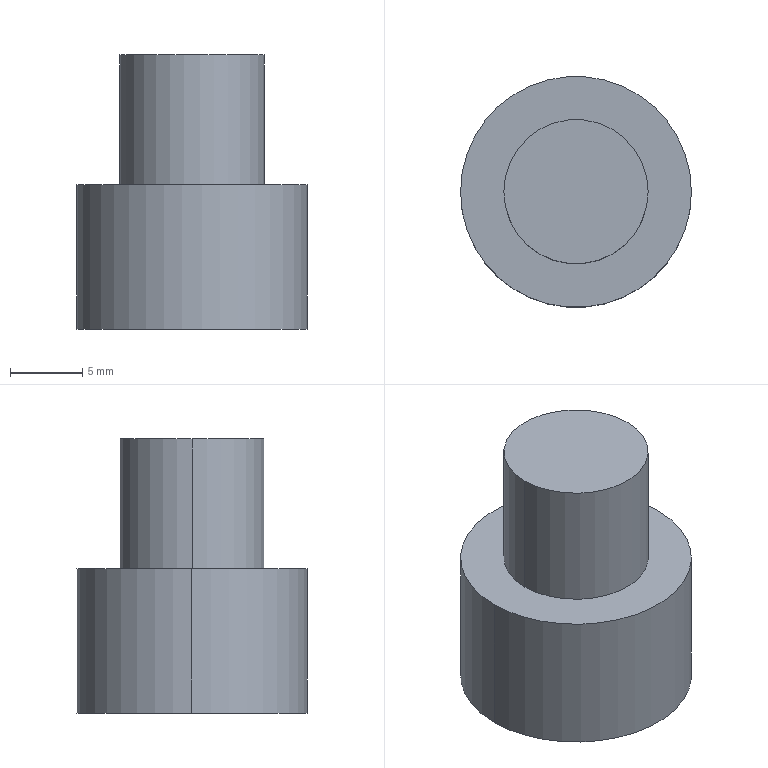Part | STEP file | LG M10_1F | 1 solid | 14 faces | box 16 x 16 x 19 mm | volume 2438 mm3 | plane 10 | cylinder 4 | commonest cylinder face diameters 10 x2 16 x2
STEP:
#1=CARTESIAN_POINT('',(0.,0.,0.));
#2=DIRECTION('',(0.,0.,1.));
#3=DIRECTION('',(1.,0.,0.));
#4=AXIS2_PLACEMENT_3D('',#1,#2,#3);
#5=CARTESIAN_POINT('',(5.,0.,9.));
#6=VERTEX_POINT('',#5);
#7=CARTESIAN_POINT('',(-5.,0.,9.));
#8=VERTEX_POINT('',#7);
#9=CARTESIAN_POINT('',(0.,0.,9.));
#10=DIRECTION('',(0.,0.,1.));
#11=DIRECTION('',(1.,0.,0.));
#12=AXIS2_PLACEMENT_3D('',#9,#10,#11);
#13=CIRCLE('',#12,5.);
#14=CARTESIAN_POINT('',(0.,0.,9.));
#15=DIRECTION('',(0.,0.,-1.));
#16=DIRECTION('',(-1.,0.,0.));
#17=AXIS2_PLACEMENT_3D('',#14,#15,#16);
#18=CYLINDRICAL_SURFACE('',#17,5.);
#19=CARTESIAN_POINT('',(3.142,0.));
#20=DIRECTION('',(-1.,0.));
#21=VECTOR('',#20,1.);
#22=LINE('',#19,#21);
#23=(GEOMETRIC_REPRESENTATION_CONTEXT(2)PARAMETRIC_REPRESENTATION_CONTEXT()REPRESENTATION_CONTEXT('',''));
#24=DEFINITIONAL_REPRESENTATION('',(#22),#23);
#25=PCURVE('',#18,#24);
#26=CARTESIAN_POINT('',(0.,0.,9.));
#27=DIRECTION('',(0.,0.,1.));
#28=DIRECTION('',(1.,0.,0.));
#29=AXIS2_PLACEMENT_3D('',#26,#27,#28);
#30=PLANE('',#29);
#31=CARTESIAN_POINT('',(0.,0.));
#32=DIRECTION('',(1.,0.));
#33=AXIS2_PLACEMENT_2D('',#31,#32);
#34=CIRCLE('',#33,5.);
#35=(GEOMETRIC_REPRESENTATION_CONTEXT(2)PARAMETRIC_REPRESENTATION_CONTEXT()REPRESENTATION_CONTEXT('',''));
#36=DEFINITIONAL_REPRESENTATION('',(#34),#35);
#37=PCURVE('',#30,#36);
#38=SURFACE_CURVE('',#13,(#25,#37),.PCURVE_S1.);
#39=EDGE_CURVE('',#6,#8,#38,.T.);
#40=ORIENTED_EDGE('',*,*,#39,.F.);
#41=CARTESIAN_POINT('',(5.,0.,0.));
#42=VERTEX_POINT('',#41);
#43=CARTESIAN_POINT('',(5.,0.,9.));
#44=DIRECTION('',(0.,0.,-1.));
#45=VECTOR('',#44,1.);
#46=LINE('',#43,#45);
#47=CARTESIAN_POINT('',(3.142,0.));
#48=DIRECTION('',(0.,1.));
#49=VECTOR('',#48,1.);
#50=LINE('',#47,#49);
#51=(GEOMETRIC_REPRESENTATION_CONTEXT(2)PARAMETRIC_REPRESENTATION_CONTEXT()REPRESENTATION_CONTEXT('',''));
#52=DEFINITIONAL_REPRESENTATION('',(#50),#51);
#53=PCURVE('',#18,#52);
#54=CARTESIAN_POINT('',(0.,0.,9.));
#55=DIRECTION('',(0.,0.,-1.));
#56=DIRECTION('',(-1.,0.,0.));
#57=AXIS2_PLACEMENT_3D('',#54,#55,#56);
#58=CYLINDRICAL_SURFACE('',#57,5.);
#59=CARTESIAN_POINT('',(3.142,0.));
#60=DIRECTION('',(0.,1.));
#61=VECTOR('',#60,1.);
#62=LINE('',#59,#61);
#63=(GEOMETRIC_REPRESENTATION_CONTEXT(2)PARAMETRIC_REPRESENTATION_CONTEXT()REPRESENTATION_CONTEXT('',''));
#64=DEFINITIONAL_REPRESENTATION('',(#62),#63);
#65=PCURVE('',#58,#64);
#66=SURFACE_CURVE('',#46,(#53,#65),.PCURVE_S1.);
#67=EDGE_CURVE('',#6,#42,#66,.T.);
#68=ORIENTED_EDGE('',*,*,#67,.T.);
#69=CARTESIAN_POINT('',(-5.,0.,0.));
#70=VERTEX_POINT('',#69);
#71=CARTESIAN_POINT('',(0.,0.,0.));
#72=DIRECTION('',(0.,0.,1.));
#73=DIRECTION('',(1.,0.,0.));
#74=AXIS2_PLACEMENT_3D('',#71,#72,#73);
#75=CIRCLE('',#74,5.);
#76=CARTESIAN_POINT('',(3.142,9.));
#77=DIRECTION('',(-1.,0.));
#78=VECTOR('',#77,1.);
#79=LINE('',#76,#78);
#80=(GEOMETRIC_REPRESENTATION_CONTEXT(2)PARAMETRIC_REPRESENTATION_CONTEXT()REPRESENTATION_CONTEXT('',''));
#81=DEFINITIONAL_REPRESENTATION('',(#79),#80);
#82=PCURVE('',#18,#81);
#83=CARTESIAN_POINT('',(0.,0.,0.));
#84=DIRECTION('',(0.,0.,1.));
#85=DIRECTION('',(1.,0.,0.));
#86=AXIS2_PLACEMENT_3D('',#83,#84,#85);
#87=PLANE('',#86);
#88=CARTESIAN_POINT('',(0.,0.));
#89=DIRECTION('',(1.,0.));
#90=AXIS2_PLACEMENT_2D('',#88,#89);
#91=CIRCLE('',#90,5.);
#92=(GEOMETRIC_REPRESENTATION_CONTEXT(2)PARAMETRIC_REPRESENTATION_CONTEXT()REPRESENTATION_CONTEXT('',''));
#93=DEFINITIONAL_REPRESENTATION('',(#91),#92);
#94=PCURVE('',#87,#93);
#95=SURFACE_CURVE('',#75,(#82,#94),.PCURVE_S1.);
#96=EDGE_CURVE('',#42,#70,#95,.T.);
#97=ORIENTED_EDGE('',*,*,#96,.T.);
#98=CARTESIAN_POINT('',(-5.,0.,9.));
#99=DIRECTION('',(0.,0.,-1.));
#100=VECTOR('',#99,1.);
#101=LINE('',#98,#100);
#102=CARTESIAN_POINT('',(0.,0.));
#103=DIRECTION('',(0.,1.));
#104=VECTOR('',#103,1.);
#105=LINE('',#102,#104);
#106=(GEOMETRIC_REPRESENTATION_CONTEXT(2)PARAMETRIC_REPRESENTATION_CONTEXT()REPRESENTATION_CONTEXT('',''));
#107=DEFINITIONAL_REPRESENTATION('',(#105),#106);
#108=PCURVE('',#18,#107);
#109=CARTESIAN_POINT('',(6.283,0.));
#110=DIRECTION('',(0.,1.));
#111=VECTOR('',#110,1.);
#112=LINE('',#109,#111);
#113=(GEOMETRIC_REPRESENTATION_CONTEXT(2)PARAMETRIC_REPRESENTATION_CONTEXT()REPRESENTATION_CONTEXT('',''));
#114=DEFINITIONAL_REPRESENTATION('',(#112),#113);
#115=PCURVE('',#58,#114);
#116=SURFACE_CURVE('',#101,(#108,#115),.PCURVE_S1.);
#117=EDGE_CURVE('',#8,#70,#116,.T.);
#118=ORIENTED_EDGE('',*,*,#117,.F.);
#119=EDGE_LOOP('',(#40,#68,#97,#118));
#120=FACE_BOUND('',#119,.T.);
#121=ADVANCED_FACE('',(#120),#18,.T.);
#122=CARTESIAN_POINT('',(8.,0.,-10.));
#123=VERTEX_POINT('',#122);
#124=CARTESIAN_POINT('',(-8.,0.,-10.));
#125=VERTEX_POINT('',#124);
#126=CARTESIAN_POINT('',(0.,0.,-10.));
#127=DIRECTION('',(0.,0.,1.));
#128=DIRECTION('',(1.,0.,0.));
#129=AXIS2_PLACEMENT_3D('',#126,#127,#128);
#130=CIRCLE('',#129,8.);
#131=CARTESIAN_POINT('',(0.,0.,-10.));
#132=DIRECTION('',(0.,0.,1.));
#133=DIRECTION('',(1.,0.,0.));
#134=AXIS2_PLACEMENT_3D('',#131,#132,#133);
#135=CYLINDRICAL_SURFACE('',#134,8.);
#136=CARTESIAN_POINT('',(0.,0.));
#137=DIRECTION('',(1.,0.));
#138=VECTOR('',#137,1.);
#139=LINE('',#136,#138);
#140=(GEOMETRIC_REPRESENTATION_CONTEXT(2)PARAMETRIC_REPRESENTATION_CONTEXT()REPRESENTATION_CONTEXT('',''));
#141=DEFINITIONAL_REPRESENTATION('',(#139),#140);
#142=PCURVE('',#135,#141);
#143=CARTESIAN_POINT('',(0.,0.,-10.));
#144=DIRECTION('',(0.,0.,1.));
#145=DIRECTION('',(1.,0.,0.));
#146=AXIS2_PLACEMENT_3D('',#143,#144,#145);
#147=PLANE('',#146);
#148=CARTESIAN_POINT('',(0.,0.));
#149=DIRECTION('',(1.,0.));
#150=AXIS2_PLACEMENT_2D('',#148,#149);
#151=CIRCLE('',#150,8.);
#152=(GEOMETRIC_REPRESENTATION_CONTEXT(2)PARAMETRIC_REPRESENTATION_CONTEXT()REPRESENTATION_CONTEXT('',''));
#153=DEFINITIONAL_REPRESENTATION('',(#151),#152);
#154=PCURVE('',#147,#153);
#155=SURFACE_CURVE('',#130,(#142,#154),.PCURVE_S1.);
#156=EDGE_CURVE('',#123,#125,#155,.T.);
#157=ORIENTED_EDGE('',*,*,#156,.T.);
#158=CARTESIAN_POINT('',(-8.,0.,0.));
#159=VERTEX_POINT('',#158);
#160=CARTESIAN_POINT('',(-8.,0.,-10.));
#161=DIRECTION('',(0.,0.,1.));
#162=VECTOR('',#161,1.);
#163=LINE('',#160,#162);
#164=CARTESIAN_POINT('',(3.142,0.));
#165=DIRECTION('',(0.,1.));
#166=VECTOR('',#165,1.);
#167=LINE('',#164,#166);
#168=(GEOMETRIC_REPRESENTATION_CONTEXT(2)PARAMETRIC_REPRESENTATION_CONTEXT()REPRESENTATION_CONTEXT('',''));
#169=DEFINITIONAL_REPRESENTATION('',(#167),#168);
#170=PCURVE('',#135,#169);
#171=CARTESIAN_POINT('',(0.,0.,-10.));
#172=DIRECTION('',(0.,0.,1.));
#173=DIRECTION('',(1.,0.,0.));
#174=AXIS2_PLACEMENT_3D('',#171,#172,#173);
#175=CYLINDRICAL_SURFACE('',#174,8.);
#176=CARTESIAN_POINT('',(3.142,0.));
#177=DIRECTION('',(0.,1.));
#178=VECTOR('',#177,1.);
#179=LINE('',#176,#178);
#180=(GEOMETRIC_REPRESENTATION_CONTEXT(2)PARAMETRIC_REPRESENTATION_CONTEXT()REPRESENTATION_CONTEXT('',''));
#181=DEFINITIONAL_REPRESENTATION('',(#179),#180);
#182=PCURVE('',#175,#181);
#183=SURFACE_CURVE('',#163,(#170,#182),.PCURVE_S1.);
#184=EDGE_CURVE('',#125,#159,#183,.T.);
#185=ORIENTED_EDGE('',*,*,#184,.T.);
#186=CARTESIAN_POINT('',(8.,0.,0.));
#187=VERTEX_POINT('',#186);
#188=CARTESIAN_POINT('',(0.,0.,0.));
#189=DIRECTION('',(0.,0.,1.));
#190=DIRECTION('',(1.,0.,0.));
#191=AXIS2_PLACEMENT_3D('',#188,#189,#190);
#192=CIRCLE('',#191,8.);
#193=CARTESIAN_POINT('',(0.,10.));
#194=DIRECTION('',(1.,0.));
#195=VECTOR('',#194,1.);
#196=LINE('',#193,#195);
#197=(GEOMETRIC_REPRESENTATION_CONTEXT(2)PARAMETRIC_REPRESENTATION_CONTEXT()REPRESENTATION_CONTEXT('',''));
#198=DEFINITIONAL_REPRESENTATION('',(#196),#197);
#199=PCURVE('',#135,#198);
#200=CARTESIAN_POINT('',(0.,0.));
#201=DIRECTION('',(1.,0.));
#202=AXIS2_PLACEMENT_2D('',#200,#201);
#203=CIRCLE('',#202,8.);
#204=(GEOMETRIC_REPRESENTATION_CONTEXT(2)PARAMETRIC_REPRESENTATION_CONTEXT()REPRESENTATION_CONTEXT('',''));
#205=DEFINITIONAL_REPRESENTATION('',(#203),#204);
#206=PCURVE('',#87,#205);
#207=SURFACE_CURVE('',#192,(#199,#206),.PCURVE_S1.);
#208=EDGE_CURVE('',#187,#159,#207,.T.);
#209=ORIENTED_EDGE('',*,*,#208,.F.);
#210=CARTESIAN_POINT('',(8.,0.,-10.));
#211=DIRECTION('',(0.,0.,1.));
#212=VECTOR('',#211,1.);
#213=LINE('',#210,#212);
#214=CARTESIAN_POINT('',(0.,0.));
#215=DIRECTION('',(0.,1.));
#216=VECTOR('',#215,1.);
#217=LINE('',#214,#216);
#218=(GEOMETRIC_REPRESENTATION_CONTEXT(2)PARAMETRIC_REPRESENTATION_CONTEXT()REPRESENTATION_CONTEXT('',''));
#219=DEFINITIONAL_REPRESENTATION('',(#217),#218);
#220=PCURVE('',#135,#219);
#221=CARTESIAN_POINT('',(6.283,0.));
#222=DIRECTION('',(0.,1.));
#223=VECTOR('',#222,1.);
#224=LINE('',#221,#223);
#225=(GEOMETRIC_REPRESENTATION_CONTEXT(2)PARAMETRIC_REPRESENTATION_CONTEXT()REPRESENTATION_CONTEXT('',''));
#226=DEFINITIONAL_REPRESENTATION('',(#224),#225);
#227=PCURVE('',#175,#226);
#228=SURFACE_CURVE('',#213,(#220,#227),.PCURVE_S1.);
#229=EDGE_CURVE('',#123,#187,#228,.T.);
#230=ORIENTED_EDGE('',*,*,#229,.F.);
#231=EDGE_LOOP('',(#157,#185,#209,#230));
#232=FACE_BOUND('',#231,.T.);
#233=ADVANCED_FACE('',(#232),#135,.T.);
#234=ORIENTED_EDGE('',*,*,#208,.T.);
#235=CARTESIAN_POINT('',(0.,0.,0.));
#236=DIRECTION('',(0.,0.,1.));
#237=DIRECTION('',(1.,0.,0.));
#238=AXIS2_PLACEMENT_3D('',#235,#236,#237);
#239=CIRCLE('',#238,8.);
#240=CARTESIAN_POINT('',(0.,0.));
#241=DIRECTION('',(1.,0.));
#242=AXIS2_PLACEMENT_2D('',#240,#241);
#243=CIRCLE('',#242,8.);
#244=(GEOMETRIC_REPRESENTATION_CONTEXT(2)PARAMETRIC_REPRESENTATION_CONTEXT()REPRESENTATION_CONTEXT('',''));
#245=DEFINITIONAL_REPRESENTATION('',(#243),#244);
#246=PCURVE('',#87,#245);
#247=CARTESIAN_POINT('',(0.,10.));
#248=DIRECTION('',(1.,0.));
#249=VECTOR('',#248,1.);
#250=LINE('',#247,#249);
#251=(GEOMETRIC_REPRESENTATION_CONTEXT(2)PARAMETRIC_REPRESENTATION_CONTEXT()REPRESENTATION_CONTEXT('',''));
#252=DEFINITIONAL_REPRESENTATION('',(#250),#251);
#253=PCURVE('',#175,#252);
#254=SURFACE_CURVE('',#239,(#246,#253),.PCURVE_S1.);
#255=EDGE_CURVE('',#159,#187,#254,.T.);
#256=ORIENTED_EDGE('',*,*,#255,.T.);
#257=EDGE_LOOP('',(#234,#256));
#258=FACE_BOUND('',#257,.T.);
#259=CARTESIAN_POINT('',(0.,0.,0.));
#260=DIRECTION('',(0.,0.,1.));
#261=DIRECTION('',(1.,0.,0.));
#262=AXIS2_PLACEMENT_3D('',#259,#260,#261);
#263=CIRCLE('',#262,5.);
#264=CARTESIAN_POINT('',(0.,0.));
#265=DIRECTION('',(1.,0.));
#266=AXIS2_PLACEMENT_2D('',#264,#265);
#267=CIRCLE('',#266,5.);
#268=(GEOMETRIC_REPRESENTATION_CONTEXT(2)PARAMETRIC_REPRESENTATION_CONTEXT()REPRESENTATION_CONTEXT('',''));
#269=DEFINITIONAL_REPRESENTATION('',(#267),#268);
#270=PCURVE('',#87,#269);
#271=CARTESIAN_POINT('',(9.425,9.));
#272=DIRECTION('',(-1.,0.));
#273=VECTOR('',#272,1.);
#274=LINE('',#271,#273);
#275=(GEOMETRIC_REPRESENTATION_CONTEXT(2)PARAMETRIC_REPRESENTATION_CONTEXT()REPRESENTATION_CONTEXT('',''));
#276=DEFINITIONAL_REPRESENTATION('',(#274),#275);
#277=PCURVE('',#58,#276);
#278=SURFACE_CURVE('',#263,(#270,#277),.PCURVE_S1.);
#279=EDGE_CURVE('',#70,#42,#278,.T.);
#280=ORIENTED_EDGE('',*,*,#279,.F.);
#281=ORIENTED_EDGE('',*,*,#96,.F.);
#282=EDGE_LOOP('',(#280,#281));
#283=FACE_BOUND('',#282,.T.);
#284=ADVANCED_FACE('',(#258,#283),#87,.T.);
#285=ORIENTED_EDGE('',*,*,#184,.F.);
#286=CARTESIAN_POINT('',(0.,0.,-10.));
#287=DIRECTION('',(0.,0.,1.));
#288=DIRECTION('',(1.,0.,0.));
#289=AXIS2_PLACEMENT_3D('',#286,#287,#288);
#290=CIRCLE('',#289,8.);
#291=CARTESIAN_POINT('',(0.,0.));
#292=DIRECTION('',(1.,0.));
#293=VECTOR('',#292,1.);
#294=LINE('',#291,#293);
#295=(GEOMETRIC_REPRESENTATION_CONTEXT(2)PARAMETRIC_REPRESENTATION_CONTEXT()REPRESENTATION_CONTEXT('',''));
#296=DEFINITIONAL_REPRESENTATION('',(#294),#295);
#297=PCURVE('',#175,#296);
#298=CARTESIAN_POINT('',(0.,0.));
#299=DIRECTION('',(1.,0.));
#300=AXIS2_PLACEMENT_2D('',#298,#299);
#301=CIRCLE('',#300,8.);
#302=(GEOMETRIC_REPRESENTATION_CONTEXT(2)PARAMETRIC_REPRESENTATION_CONTEXT()REPRESENTATION_CONTEXT('',''));
#303=DEFINITIONAL_REPRESENTATION('',(#301),#302);
#304=PCURVE('',#147,#303);
#305=SURFACE_CURVE('',#290,(#297,#304),.PCURVE_S1.);
#306=EDGE_CURVE('',#125,#123,#305,.T.);
#307=ORIENTED_EDGE('',*,*,#306,.T.);
#308=ORIENTED_EDGE('',*,*,#229,.T.);
#309=ORIENTED_EDGE('',*,*,#255,.F.);
#310=EDGE_LOOP('',(#285,#307,#308,#309));
#311=FACE_BOUND('',#310,.T.);
#312=ADVANCED_FACE('',(#311),#175,.T.);
#313=CARTESIAN_POINT('',(-4.636,0.,-10.));
#314=VERTEX_POINT('',#313);
#315=CARTESIAN_POINT('',(-2.318,4.015,-10.));
#316=VERTEX_POINT('',#315);
#317=CARTESIAN_POINT('',(-4.636,0.,-10.));
#318=DIRECTION('',(0.5,0.866,0.));
#319=VECTOR('',#318,1.);
#320=LINE('',#317,#319);
#321=CARTESIAN_POINT('',(-4.636,0.));
#322=DIRECTION('',(0.5,0.866));
#323=VECTOR('',#322,1.);
#324=LINE('',#321,#323);
#325=(GEOMETRIC_REPRESENTATION_CONTEXT(2)PARAMETRIC_REPRESENTATION_CONTEXT()REPRESENTATION_CONTEXT('',''));
#326=DEFINITIONAL_REPRESENTATION('',(#324),#325);
#327=PCURVE('',#147,#326);
#328=CARTESIAN_POINT('',(-4.636,0.,-5.));
#329=DIRECTION('',(-0.866,0.5,0.));
#330=DIRECTION('',(-0.5,-0.866,0.));
#331=AXIS2_PLACEMENT_3D('',#328,#329,#330);
#332=PLANE('',#331);
#333=CARTESIAN_POINT('',(0.,-5.));
#334=DIRECTION('',(-1.,0.));
#335=VECTOR('',#334,1.);
#336=LINE('',#333,#335);
#337=(GEOMETRIC_REPRESENTATION_CONTEXT(2)PARAMETRIC_REPRESENTATION_CONTEXT()REPRESENTATION_CONTEXT('',''));
#338=DEFINITIONAL_REPRESENTATION('',(#336),#337);
#339=PCURVE('',#332,#338);
#340=SURFACE_CURVE('',#320,(#327,#339),.PCURVE_S1.);
#341=EDGE_CURVE('',#314,#316,#340,.T.);
#342=ORIENTED_EDGE('',*,*,#341,.F.);
#343=CARTESIAN_POINT('',(-2.318,-4.015,-10.));
#344=VERTEX_POINT('',#343);
#345=CARTESIAN_POINT('',(-2.318,-4.015,-10.));
#346=DIRECTION('',(-0.5,0.866,0.));
#347=VECTOR('',#346,1.);
#348=LINE('',#345,#347);
#349=CARTESIAN_POINT('',(-2.318,-4.015));
#350=DIRECTION('',(-0.5,0.866));
#351=VECTOR('',#350,1.);
#352=LINE('',#349,#351);
#353=(GEOMETRIC_REPRESENTATION_CONTEXT(2)PARAMETRIC_REPRESENTATION_CONTEXT()REPRESENTATION_CONTEXT('',''));
#354=DEFINITIONAL_REPRESENTATION('',(#352),#353);
#355=PCURVE('',#147,#354);
#356=CARTESIAN_POINT('',(-2.318,-4.015,-5.));
#357=DIRECTION('',(-0.866,-0.5,0.));
#358=DIRECTION('',(0.5,-0.866,0.));
#359=AXIS2_PLACEMENT_3D('',#356,#357,#358);
#360=PLANE('',#359);
#361=CARTESIAN_POINT('',(0.,-5.));
#362=DIRECTION('',(-1.,0.));
#363=VECTOR('',#362,1.);
#364=LINE('',#361,#363);
#365=(GEOMETRIC_REPRESENTATION_CONTEXT(2)PARAMETRIC_REPRESENTATION_CONTEXT()REPRESENTATION_CONTEXT('',''));
#366=DEFINITIONAL_REPRESENTATION('',(#364),#365);
#367=PCURVE('',#360,#366);
#368=SURFACE_CURVE('',#348,(#355,#367),.PCURVE_S1.);
#369=EDGE_CURVE('',#344,#314,#368,.T.);
#370=ORIENTED_EDGE('',*,*,#369,.F.);
#371=CARTESIAN_POINT('',(2.318,-4.015,-10.));
#372=VERTEX_POINT('',#371);
#373=CARTESIAN_POINT('',(2.318,-4.015,-10.));
#374=DIRECTION('',(-1.,0.,0.));
#375=VECTOR('',#374,1.);
#376=LINE('',#373,#375);
#377=CARTESIAN_POINT('',(2.318,-4.015));
#378=DIRECTION('',(-1.,0.));
#379=VECTOR('',#378,1.);
#380=LINE('',#377,#379);
#381=(GEOMETRIC_REPRESENTATION_CONTEXT(2)PARAMETRIC_REPRESENTATION_CONTEXT()REPRESENTATION_CONTEXT('',''));
#382=DEFINITIONAL_REPRESENTATION('',(#380),#381);
#383=PCURVE('',#147,#382);
#384=CARTESIAN_POINT('',(2.318,-4.015,-5.));
#385=DIRECTION('',(0.,-1.,0.));
#386=DIRECTION('',(1.,0.,0.));
#387=AXIS2_PLACEMENT_3D('',#384,#385,#386);
#388=PLANE('',#387);
#389=CARTESIAN_POINT('',(0.,-5.));
#390=DIRECTION('',(-1.,0.));
#391=VECTOR('',#390,1.);
#392=LINE('',#389,#391);
#393=(GEOMETRIC_REPRESENTATION_CONTEXT(2)PARAMETRIC_REPRESENTATION_CONTEXT()REPRESENTATION_CONTEXT('',''));
#394=DEFINITIONAL_REPRESENTATION('',(#392),#393);
#395=PCURVE('',#388,#394);
#396=SURFACE_CURVE('',#376,(#383,#395),.PCURVE_S1.);
#397=EDGE_CURVE('',#372,#344,#396,.T.);
#398=ORIENTED_EDGE('',*,*,#397,.F.);
#399=CARTESIAN_POINT('',(4.636,0.,-10.));
#400=VERTEX_POINT('',#399);
#401=CARTESIAN_POINT('',(4.636,0.,-10.));
#402=DIRECTION('',(-0.5,-0.866,0.));
#403=VECTOR('',#402,1.);
#404=LINE('',#401,#403);
#405=CARTESIAN_POINT('',(4.636,0.));
#406=DIRECTION('',(-0.5,-0.866));
#407=VECTOR('',#406,1.);
#408=LINE('',#405,#407);
#409=(GEOMETRIC_REPRESENTATION_CONTEXT(2)PARAMETRIC_REPRESENTATION_CONTEXT()REPRESENTATION_CONTEXT('',''));
#410=DEFINITIONAL_REPRESENTATION('',(#408),#409);
#411=PCURVE('',#147,#410);
#412=CARTESIAN_POINT('',(4.636,0.,-5.));
#413=DIRECTION('',(0.866,-0.5,0.));
#414=DIRECTION('',(0.5,0.866,0.));
#415=AXIS2_PLACEMENT_3D('',#412,#413,#414);
#416=PLANE('',#415);
#417=CARTESIAN_POINT('',(0.,-5.));
#418=DIRECTION('',(-1.,0.));
#419=VECTOR('',#418,1.);
#420=LINE('',#417,#419);
#421=(GEOMETRIC_REPRESENTATION_CONTEXT(2)PARAMETRIC_REPRESENTATION_CONTEXT()REPRESENTATION_CONTEXT('',''));
#422=DEFINITIONAL_REPRESENTATION('',(#420),#421);
#423=PCURVE('',#416,#422);
#424=SURFACE_CURVE('',#404,(#411,#423),.PCURVE_S1.);
#425=EDGE_CURVE('',#400,#372,#424,.T.);
#426=ORIENTED_EDGE('',*,*,#425,.F.);
#427=CARTESIAN_POINT('',(2.318,4.015,-10.));
#428=VERTEX_POINT('',#427);
#429=CARTESIAN_POINT('',(2.318,4.015,-10.));
#430=DIRECTION('',(0.5,-0.866,0.));
#431=VECTOR('',#430,1.);
#432=LINE('',#429,#431);
#433=CARTESIAN_POINT('',(2.318,4.015));
#434=DIRECTION('',(0.5,-0.866));
#435=VECTOR('',#434,1.);
#436=LINE('',#433,#435);
#437=(GEOMETRIC_REPRESENTATION_CONTEXT(2)PARAMETRIC_REPRESENTATION_CONTEXT()REPRESENTATION_CONTEXT('',''));
#438=DEFINITIONAL_REPRESENTATION('',(#436),#437);
#439=PCURVE('',#147,#438);
#440=CARTESIAN_POINT('',(2.318,4.015,-5.));
#441=DIRECTION('',(0.866,0.5,0.));
#442=DIRECTION('',(-0.5,0.866,0.));
#443=AXIS2_PLACEMENT_3D('',#440,#441,#442);
#444=PLANE('',#443);
#445=CARTESIAN_POINT('',(0.,-5.));
#446=DIRECTION('',(-1.,0.));
#447=VECTOR('',#446,1.);
#448=LINE('',#445,#447);
#449=(GEOMETRIC_REPRESENTATION_CONTEXT(2)PARAMETRIC_REPRESENTATION_CONTEXT()REPRESENTATION_CONTEXT('',''));
#450=DEFINITIONAL_REPRESENTATION('',(#448),#449);
#451=PCURVE('',#444,#450);
#452=SURFACE_CURVE('',#432,(#439,#451),.PCURVE_S1.);
#453=EDGE_CURVE('',#428,#400,#452,.T.);
#454=ORIENTED_EDGE('',*,*,#453,.F.);
#455=CARTESIAN_POINT('',(-2.318,4.015,-10.));
#456=DIRECTION('',(1.,0.,0.));
#457=VECTOR('',#456,1.);
#458=LINE('',#455,#457);
#459=CARTESIAN_POINT('',(-2.318,4.015));
#460=DIRECTION('',(1.,0.));
#461=VECTOR('',#460,1.);
#462=LINE('',#459,#461);
#463=(GEOMETRIC_REPRESENTATION_CONTEXT(2)PARAMETRIC_REPRESENTATION_CONTEXT()REPRESENTATION_CONTEXT('',''));
#464=DEFINITIONAL_REPRESENTATION('',(#462),#463);
#465=PCURVE('',#147,#464);
#466=CARTESIAN_POINT('',(-2.318,4.015,-5.));
#467=DIRECTION('',(0.,1.,0.));
#468=DIRECTION('',(-1.,0.,0.));
#469=AXIS2_PLACEMENT_3D('',#466,#467,#468);
#470=PLANE('',#469);
#471=CARTESIAN_POINT('',(0.,-5.));
#472=DIRECTION('',(-1.,0.));
#473=VECTOR('',#472,1.);
#474=LINE('',#471,#473);
#475=(GEOMETRIC_REPRESENTATION_CONTEXT(2)PARAMETRIC_REPRESENTATION_CONTEXT()REPRESENTATION_CONTEXT('',''));
#476=DEFINITIONAL_REPRESENTATION('',(#474),#475);
#477=PCURVE('',#470,#476);
#478=SURFACE_CURVE('',#458,(#465,#477),.PCURVE_S1.);
#479=EDGE_CURVE('',#316,#428,#478,.T.);
#480=ORIENTED_EDGE('',*,*,#479,.F.);
#481=EDGE_LOOP('',(#342,#370,#398,#426,#454,#480));
#482=FACE_BOUND('',#481,.T.);
#483=ORIENTED_EDGE('',*,*,#156,.F.);
#484=ORIENTED_EDGE('',*,*,#306,.F.);
#485=EDGE_LOOP('',(#483,#484));
#486=FACE_BOUND('',#485,.T.);
#487=ADVANCED_FACE('',(#482,#486),#147,.F.);
#488=ORIENTED_EDGE('',*,*,#67,.F.);
#489=CARTESIAN_POINT('',(0.,0.,9.));
#490=DIRECTION('',(0.,0.,1.));
#491=DIRECTION('',(1.,0.,0.));
#492=AXIS2_PLACEMENT_3D('',#489,#490,#491);
#493=CIRCLE('',#492,5.);
#494=CARTESIAN_POINT('',(9.425,0.));
#495=DIRECTION('',(-1.,0.));
#496=VECTOR('',#495,1.);
#497=LINE('',#494,#496);
#498=(GEOMETRIC_REPRESENTATION_CONTEXT(2)PARAMETRIC_REPRESENTATION_CONTEXT()REPRESENTATION_CONTEXT('',''));
#499=DEFINITIONAL_REPRESENTATION('',(#497),#498);
#500=PCURVE('',#58,#499);
#501=CARTESIAN_POINT('',(0.,0.));
#502=DIRECTION('',(1.,0.));
#503=AXIS2_PLACEMENT_2D('',#501,#502);
#504=CIRCLE('',#503,5.);
#505=(GEOMETRIC_REPRESENTATION_CONTEXT(2)PARAMETRIC_REPRESENTATION_CONTEXT()REPRESENTATION_CONTEXT('',''));
#506=DEFINITIONAL_REPRESENTATION('',(#504),#505);
#507=PCURVE('',#30,#506);
#508=SURFACE_CURVE('',#493,(#500,#507),.PCURVE_S1.);
#509=EDGE_CURVE('',#8,#6,#508,.T.);
#510=ORIENTED_EDGE('',*,*,#509,.F.);
#511=ORIENTED_EDGE('',*,*,#117,.T.);
#512=ORIENTED_EDGE('',*,*,#279,.T.);
#513=EDGE_LOOP('',(#488,#510,#511,#512));
#514=FACE_BOUND('',#513,.T.);
#515=ADVANCED_FACE('',(#514),#58,.T.);
#516=ORIENTED_EDGE('',*,*,#509,.T.);
#517=ORIENTED_EDGE('',*,*,#39,.T.);
#518=EDGE_LOOP('',(#516,#517));
#519=FACE_BOUND('',#518,.T.);
#520=ADVANCED_FACE('',(#519),#30,.T.);
#521=ORIENTED_EDGE('',*,*,#369,.T.);
#522=CARTESIAN_POINT('',(-4.636,0.,-5.));
#523=VERTEX_POINT('',#522);
#524=CARTESIAN_POINT('',(-4.636,0.,-5.));
#525=DIRECTION('',(0.,0.,-1.));
#526=VECTOR('',#525,1.);
#527=LINE('',#524,#526);
#528=CARTESIAN_POINT('',(-4.636,0.));
#529=DIRECTION('',(0.,-1.));
#530=VECTOR('',#529,1.);
#531=LINE('',#528,#530);
#532=(GEOMETRIC_REPRESENTATION_CONTEXT(2)PARAMETRIC_REPRESENTATION_CONTEXT()REPRESENTATION_CONTEXT('',''));
#533=DEFINITIONAL_REPRESENTATION('',(#531),#532);
#534=PCURVE('',#360,#533);
#535=CARTESIAN_POINT('',(0.,0.));
#536=DIRECTION('',(0.,-1.));
#537=VECTOR('',#536,1.);
#538=LINE('',#535,#537);
#539=(GEOMETRIC_REPRESENTATION_CONTEXT(2)PARAMETRIC_REPRESENTATION_CONTEXT()REPRESENTATION_CONTEXT('',''));
#540=DEFINITIONAL_REPRESENTATION('',(#538),#539);
#541=PCURVE('',#332,#540);
#542=SURFACE_CURVE('',#527,(#534,#541),.PCURVE_S1.);
#543=EDGE_CURVE('',#523,#314,#542,.T.);
#544=ORIENTED_EDGE('',*,*,#543,.F.);
#545=CARTESIAN_POINT('',(-2.318,-4.015,-5.));
#546=VERTEX_POINT('',#545);
#547=CARTESIAN_POINT('',(-2.318,-4.015,-5.));
#548=DIRECTION('',(-0.5,0.866,0.));
#549=VECTOR('',#548,1.);
#550=LINE('',#547,#549);
#551=CARTESIAN_POINT('',(0.,0.));
#552=DIRECTION('',(-1.,0.));
#553=VECTOR('',#552,1.);
#554=LINE('',#551,#553);
#555=(GEOMETRIC_REPRESENTATION_CONTEXT(2)PARAMETRIC_REPRESENTATION_CONTEXT()REPRESENTATION_CONTEXT('',''));
#556=DEFINITIONAL_REPRESENTATION('',(#554),#555);
#557=PCURVE('',#360,#556);
#558=CARTESIAN_POINT('',(0.,0.,-5.));
#559=DIRECTION('',(0.,0.,-1.));
#560=DIRECTION('',(-1.,0.,0.));
#561=AXIS2_PLACEMENT_3D('',#558,#559,#560);
#562=PLANE('',#561);
#563=CARTESIAN_POINT('',(2.318,-4.015));
#564=DIRECTION('',(0.5,0.866));
#565=VECTOR('',#564,1.);
#566=LINE('',#563,#565);
#567=(GEOMETRIC_REPRESENTATION_CONTEXT(2)PARAMETRIC_REPRESENTATION_CONTEXT()REPRESENTATION_CONTEXT('',''));
#568=DEFINITIONAL_REPRESENTATION('',(#566),#567);
#569=PCURVE('',#562,#568);
#570=SURFACE_CURVE('',#550,(#557,#569),.PCURVE_S1.);
#571=EDGE_CURVE('',#546,#523,#570,.T.);
#572=ORIENTED_EDGE('',*,*,#571,.F.);
#573=CARTESIAN_POINT('',(-2.318,-4.015,-5.));
#574=DIRECTION('',(0.,0.,-1.));
#575=VECTOR('',#574,1.);
#576=LINE('',#573,#575);
#577=CARTESIAN_POINT('',(0.,0.));
#578=DIRECTION('',(0.,-1.));
#579=VECTOR('',#578,1.);
#580=LINE('',#577,#579);
#581=(GEOMETRIC_REPRESENTATION_CONTEXT(2)PARAMETRIC_REPRESENTATION_CONTEXT()REPRESENTATION_CONTEXT('',''));
#582=DEFINITIONAL_REPRESENTATION('',(#580),#581);
#583=PCURVE('',#360,#582);
#584=CARTESIAN_POINT('',(-4.636,0.));
#585=DIRECTION('',(0.,-1.));
#586=VECTOR('',#585,1.);
#587=LINE('',#584,#586);
#588=(GEOMETRIC_REPRESENTATION_CONTEXT(2)PARAMETRIC_REPRESENTATION_CONTEXT()REPRESENTATION_CONTEXT('',''));
#589=DEFINITIONAL_REPRESENTATION('',(#587),#588);
#590=PCURVE('',#388,#589);
#591=SURFACE_CURVE('',#576,(#583,#590),.PCURVE_S1.);
#592=EDGE_CURVE('',#546,#344,#591,.T.);
#593=ORIENTED_EDGE('',*,*,#592,.T.);
#594=EDGE_LOOP('',(#521,#544,#572,#593));
#595=FACE_BOUND('',#594,.T.);
#596=ADVANCED_FACE('',(#595),#360,.F.);
#597=ORIENTED_EDGE('',*,*,#397,.T.);
#598=ORIENTED_EDGE('',*,*,#592,.F.);
#599=CARTESIAN_POINT('',(2.318,-4.015,-5.));
#600=VERTEX_POINT('',#599);
#601=CARTESIAN_POINT('',(2.318,-4.015,-5.));
#602=DIRECTION('',(-1.,0.,0.));
#603=VECTOR('',#602,1.);
#604=LINE('',#601,#603);
#605=CARTESIAN_POINT('',(0.,0.));
#606=DIRECTION('',(-1.,0.));
#607=VECTOR('',#606,1.);
#608=LINE('',#605,#607);
#609=(GEOMETRIC_REPRESENTATION_CONTEXT(2)PARAMETRIC_REPRESENTATION_CONTEXT()REPRESENTATION_CONTEXT('',''));
#610=DEFINITIONAL_REPRESENTATION('',(#608),#609);
#611=PCURVE('',#388,#610);
#612=CARTESIAN_POINT('',(-2.318,-4.015));
#613=DIRECTION('',(1.,0.));
#614=VECTOR('',#613,1.);
#615=LINE('',#612,#614);
#616=(GEOMETRIC_REPRESENTATION_CONTEXT(2)PARAMETRIC_REPRESENTATION_CONTEXT()REPRESENTATION_CONTEXT('',''));
#617=DEFINITIONAL_REPRESENTATION('',(#615),#616);
#618=PCURVE('',#562,#617);
#619=SURFACE_CURVE('',#604,(#611,#618),.PCURVE_S1.);
#620=EDGE_CURVE('',#600,#546,#619,.T.);
#621=ORIENTED_EDGE('',*,*,#620,.F.);
#622=CARTESIAN_POINT('',(2.318,-4.015,-5.));
#623=DIRECTION('',(0.,0.,-1.));
#624=VECTOR('',#623,1.);
#625=LINE('',#622,#624);
#626=CARTESIAN_POINT('',(0.,0.));
#627=DIRECTION('',(0.,-1.));
#628=VECTOR('',#627,1.);
#629=LINE('',#626,#628);
#630=(GEOMETRIC_REPRESENTATION_CONTEXT(2)PARAMETRIC_REPRESENTATION_CONTEXT()REPRESENTATION_CONTEXT('',''));
#631=DEFINITIONAL_REPRESENTATION('',(#629),#630);
#632=PCURVE('',#388,#631);
#633=CARTESIAN_POINT('',(-4.636,0.));
#634=DIRECTION('',(0.,-1.));
#635=VECTOR('',#634,1.);
#636=LINE('',#633,#635);
#637=(GEOMETRIC_REPRESENTATION_CONTEXT(2)PARAMETRIC_REPRESENTATION_CONTEXT()REPRESENTATION_CONTEXT('',''));
#638=DEFINITIONAL_REPRESENTATION('',(#636),#637);
#639=PCURVE('',#416,#638);
#640=SURFACE_CURVE('',#625,(#632,#639),.PCURVE_S1.);
#641=EDGE_CURVE('',#600,#372,#640,.T.);
#642=ORIENTED_EDGE('',*,*,#641,.T.);
#643=EDGE_LOOP('',(#597,#598,#621,#642));
#644=FACE_BOUND('',#643,.T.);
#645=ADVANCED_FACE('',(#644),#388,.F.);
#646=ORIENTED_EDGE('',*,*,#425,.T.);
#647=ORIENTED_EDGE('',*,*,#641,.F.);
#648=CARTESIAN_POINT('',(4.636,0.,-5.));
#649=VERTEX_POINT('',#648);
#650=CARTESIAN_POINT('',(4.636,0.,-5.));
#651=DIRECTION('',(-0.5,-0.866,0.));
#652=VECTOR('',#651,1.);
#653=LINE('',#650,#652);
#654=CARTESIAN_POINT('',(0.,0.));
#655=DIRECTION('',(-1.,0.));
#656=VECTOR('',#655,1.);
#657=LINE('',#654,#656);
#658=(GEOMETRIC_REPRESENTATION_CONTEXT(2)PARAMETRIC_REPRESENTATION_CONTEXT()REPRESENTATION_CONTEXT('',''));
#659=DEFINITIONAL_REPRESENTATION('',(#657),#658);
#660=PCURVE('',#416,#659);
#661=CARTESIAN_POINT('',(-4.636,0.));
#662=DIRECTION('',(0.5,-0.866));
#663=VECTOR('',#662,1.);
#664=LINE('',#661,#663);
#665=(GEOMETRIC_REPRESENTATION_CONTEXT(2)PARAMETRIC_REPRESENTATION_CONTEXT()REPRESENTATION_CONTEXT('',''));
#666=DEFINITIONAL_REPRESENTATION('',(#664),#665);
#667=PCURVE('',#562,#666);
#668=SURFACE_CURVE('',#653,(#660,#667),.PCURVE_S1.);
#669=EDGE_CURVE('',#649,#600,#668,.T.);
#670=ORIENTED_EDGE('',*,*,#669,.F.);
#671=CARTESIAN_POINT('',(4.636,0.,-5.));
#672=DIRECTION('',(0.,0.,-1.));
#673=VECTOR('',#672,1.);
#674=LINE('',#671,#673);
#675=CARTESIAN_POINT('',(0.,0.));
#676=DIRECTION('',(0.,-1.));
#677=VECTOR('',#676,1.);
#678=LINE('',#675,#677);
#679=(GEOMETRIC_REPRESENTATION_CONTEXT(2)PARAMETRIC_REPRESENTATION_CONTEXT()REPRESENTATION_CONTEXT('',''));
#680=DEFINITIONAL_REPRESENTATION('',(#678),#679);
#681=PCURVE('',#416,#680);
#682=CARTESIAN_POINT('',(-4.636,0.));
#683=DIRECTION('',(0.,-1.));
#684=VECTOR('',#683,1.);
#685=LINE('',#682,#684);
#686=(GEOMETRIC_REPRESENTATION_CONTEXT(2)PARAMETRIC_REPRESENTATION_CONTEXT()REPRESENTATION_CONTEXT('',''));
#687=DEFINITIONAL_REPRESENTATION('',(#685),#686);
#688=PCURVE('',#444,#687);
#689=SURFACE_CURVE('',#674,(#681,#688),.PCURVE_S1.);
#690=EDGE_CURVE('',#649,#400,#689,.T.);
#691=ORIENTED_EDGE('',*,*,#690,.T.);
#692=EDGE_LOOP('',(#646,#647,#670,#691));
#693=FACE_BOUND('',#692,.T.);
#694=ADVANCED_FACE('',(#693),#416,.F.);
#695=ORIENTED_EDGE('',*,*,#453,.T.);
#696=ORIENTED_EDGE('',*,*,#690,.F.);
#697=CARTESIAN_POINT('',(2.318,4.015,-5.));
#698=VERTEX_POINT('',#697);
#699=CARTESIAN_POINT('',(2.318,4.015,-5.));
#700=DIRECTION('',(0.5,-0.866,0.));
#701=VECTOR('',#700,1.);
#702=LINE('',#699,#701);
#703=CARTESIAN_POINT('',(0.,0.));
#704=DIRECTION('',(-1.,0.));
#705=VECTOR('',#704,1.);
#706=LINE('',#703,#705);
#707=(GEOMETRIC_REPRESENTATION_CONTEXT(2)PARAMETRIC_REPRESENTATION_CONTEXT()REPRESENTATION_CONTEXT('',''));
#708=DEFINITIONAL_REPRESENTATION('',(#706),#707);
#709=PCURVE('',#444,#708);
#710=CARTESIAN_POINT('',(-2.318,4.015));
#711=DIRECTION('',(-0.5,-0.866));
#712=VECTOR('',#711,1.);
#713=LINE('',#710,#712);
#714=(GEOMETRIC_REPRESENTATION_CONTEXT(2)PARAMETRIC_REPRESENTATION_CONTEXT()REPRESENTATION_CONTEXT('',''));
#715=DEFINITIONAL_REPRESENTATION('',(#713),#714);
#716=PCURVE('',#562,#715);
#717=SURFACE_CURVE('',#702,(#709,#716),.PCURVE_S1.);
#718=EDGE_CURVE('',#698,#649,#717,.T.);
#719=ORIENTED_EDGE('',*,*,#718,.F.);
#720=CARTESIAN_POINT('',(2.318,4.015,-5.));
#721=DIRECTION('',(0.,0.,-1.));
#722=VECTOR('',#721,1.);
#723=LINE('',#720,#722);
#724=CARTESIAN_POINT('',(0.,0.));
#725=DIRECTION('',(0.,-1.));
#726=VECTOR('',#725,1.);
#727=LINE('',#724,#726);
#728=(GEOMETRIC_REPRESENTATION_CONTEXT(2)PARAMETRIC_REPRESENTATION_CONTEXT()REPRESENTATION_CONTEXT('',''));
#729=DEFINITIONAL_REPRESENTATION('',(#727),#728);
#730=PCURVE('',#444,#729);
#731=CARTESIAN_POINT('',(-4.636,0.));
#732=DIRECTION('',(0.,-1.));
#733=VECTOR('',#732,1.);
#734=LINE('',#731,#733);
#735=(GEOMETRIC_REPRESENTATION_CONTEXT(2)PARAMETRIC_REPRESENTATION_CONTEXT()REPRESENTATION_CONTEXT('',''));
#736=DEFINITIONAL_REPRESENTATION('',(#734),#735);
#737=PCURVE('',#470,#736);
#738=SURFACE_CURVE('',#723,(#730,#737),.PCURVE_S1.);
#739=EDGE_CURVE('',#698,#428,#738,.T.);
#740=ORIENTED_EDGE('',*,*,#739,.T.);
#741=EDGE_LOOP('',(#695,#696,#719,#740));
#742=FACE_BOUND('',#741,.T.);
#743=ADVANCED_FACE('',(#742),#444,.F.);
#744=ORIENTED_EDGE('',*,*,#479,.T.);
#745=ORIENTED_EDGE('',*,*,#739,.F.);
#746=CARTESIAN_POINT('',(-2.318,4.015,-5.));
#747=VERTEX_POINT('',#746);
#748=CARTESIAN_POINT('',(-2.318,4.015,-5.));
#749=DIRECTION('',(1.,0.,0.));
#750=VECTOR('',#749,1.);
#751=LINE('',#748,#750);
#752=CARTESIAN_POINT('',(0.,0.));
#753=DIRECTION('',(-1.,0.));
#754=VECTOR('',#753,1.);
#755=LINE('',#752,#754);
#756=(GEOMETRIC_REPRESENTATION_CONTEXT(2)PARAMETRIC_REPRESENTATION_CONTEXT()REPRESENTATION_CONTEXT('',''));
#757=DEFINITIONAL_REPRESENTATION('',(#755),#756);
#758=PCURVE('',#470,#757);
#759=CARTESIAN_POINT('',(2.318,4.015));
#760=DIRECTION('',(-1.,0.));
#761=VECTOR('',#760,1.);
#762=LINE('',#759,#761);
#763=(GEOMETRIC_REPRESENTATION_CONTEXT(2)PARAMETRIC_REPRESENTATION_CONTEXT()REPRESENTATION_CONTEXT('',''));
#764=DEFINITIONAL_REPRESENTATION('',(#762),#763);
#765=PCURVE('',#562,#764);
#766=SURFACE_CURVE('',#751,(#758,#765),.PCURVE_S1.);
#767=EDGE_CURVE('',#747,#698,#766,.T.);
#768=ORIENTED_EDGE('',*,*,#767,.F.);
#769=CARTESIAN_POINT('',(-2.318,4.015,-5.));
#770=DIRECTION('',(0.,0.,-1.));
#771=VECTOR('',#770,1.);
#772=LINE('',#769,#771);
#773=CARTESIAN_POINT('',(0.,0.));
#774=DIRECTION('',(0.,-1.));
#775=VECTOR('',#774,1.);
#776=LINE('',#773,#775);
#777=(GEOMETRIC_REPRESENTATION_CONTEXT(2)PARAMETRIC_REPRESENTATION_CONTEXT()REPRESENTATION_CONTEXT('',''));
#778=DEFINITIONAL_REPRESENTATION('',(#776),#777);
#779=PCURVE('',#470,#778);
#780=CARTESIAN_POINT('',(-4.636,0.));
#781=DIRECTION('',(0.,-1.));
#782=VECTOR('',#781,1.);
#783=LINE('',#780,#782);
#784=(GEOMETRIC_REPRESENTATION_CONTEXT(2)PARAMETRIC_REPRESENTATION_CONTEXT()REPRESENTATION_CONTEXT('',''));
#785=DEFINITIONAL_REPRESENTATION('',(#783),#784);
#786=PCURVE('',#332,#785);
#787=SURFACE_CURVE('',#772,(#779,#786),.PCURVE_S1.);
#788=EDGE_CURVE('',#747,#316,#787,.T.);
#789=ORIENTED_EDGE('',*,*,#788,.T.);
#790=EDGE_LOOP('',(#744,#745,#768,#789));
#791=FACE_BOUND('',#790,.T.);
#792=ADVANCED_FACE('',(#791),#470,.F.);
#793=ORIENTED_EDGE('',*,*,#341,.T.);
#794=ORIENTED_EDGE('',*,*,#788,.F.);
#795=CARTESIAN_POINT('',(-4.636,0.,-5.));
#796=DIRECTION('',(0.5,0.866,0.));
#797=VECTOR('',#796,1.);
#798=LINE('',#795,#797);
#799=CARTESIAN_POINT('',(0.,0.));
#800=DIRECTION('',(-1.,0.));
#801=VECTOR('',#800,1.);
#802=LINE('',#799,#801);
#803=(GEOMETRIC_REPRESENTATION_CONTEXT(2)PARAMETRIC_REPRESENTATION_CONTEXT()REPRESENTATION_CONTEXT('',''));
#804=DEFINITIONAL_REPRESENTATION('',(#802),#803);
#805=PCURVE('',#332,#804);
#806=CARTESIAN_POINT('',(4.636,0.));
#807=DIRECTION('',(-0.5,0.866));
#808=VECTOR('',#807,1.);
#809=LINE('',#806,#808);
#810=(GEOMETRIC_REPRESENTATION_CONTEXT(2)PARAMETRIC_REPRESENTATION_CONTEXT()REPRESENTATION_CONTEXT('',''));
#811=DEFINITIONAL_REPRESENTATION('',(#809),#810);
#812=PCURVE('',#562,#811);
#813=SURFACE_CURVE('',#798,(#805,#812),.PCURVE_S1.);
#814=EDGE_CURVE('',#523,#747,#813,.T.);
#815=ORIENTED_EDGE('',*,*,#814,.F.);
#816=ORIENTED_EDGE('',*,*,#543,.T.);
#817=EDGE_LOOP('',(#793,#794,#815,#816));
#818=FACE_BOUND('',#817,.T.);
#819=ADVANCED_FACE('',(#818),#332,.F.);
#820=ORIENTED_EDGE('',*,*,#571,.T.);
#821=ORIENTED_EDGE('',*,*,#814,.T.);
#822=ORIENTED_EDGE('',*,*,#767,.T.);
#823=ORIENTED_EDGE('',*,*,#718,.T.);
#824=ORIENTED_EDGE('',*,*,#669,.T.);
#825=ORIENTED_EDGE('',*,*,#620,.T.);
#826=EDGE_LOOP('',(#820,#821,#822,#823,#824,#825));
#827=FACE_BOUND('',#826,.T.);
#828=ADVANCED_FACE('',(#827),#562,.T.);
#829=CLOSED_SHELL('',(#121,#233,#284,#312,#487,#515,#520,#596,#645,#694,#743,#792,#819,#828));
#830=MANIFOLD_SOLID_BREP('',#829);
#831=(LENGTH_UNIT()NAMED_UNIT(*)SI_UNIT(.MILLI.,.METRE.));
#832=UNCERTAINTY_MEASURE_WITH_UNIT(LENGTH_MEASURE(0.0000001),#831,'','');
#833=(NAMED_UNIT(*)PLANE_ANGLE_UNIT()SI_UNIT($,.RADIAN.));
#834=(NAMED_UNIT(*)SI_UNIT($,.STERADIAN.)SOLID_ANGLE_UNIT());
#835=(GEOMETRIC_REPRESENTATION_CONTEXT(3)GLOBAL_UNCERTAINTY_ASSIGNED_CONTEXT((#832))GLOBAL_UNIT_ASSIGNED_CONTEXT((#831,#833,#834))REPRESENTATION_CONTEXT('',''));
#836=ADVANCED_BREP_SHAPE_REPRESENTATION('',(#4,#830),#835);